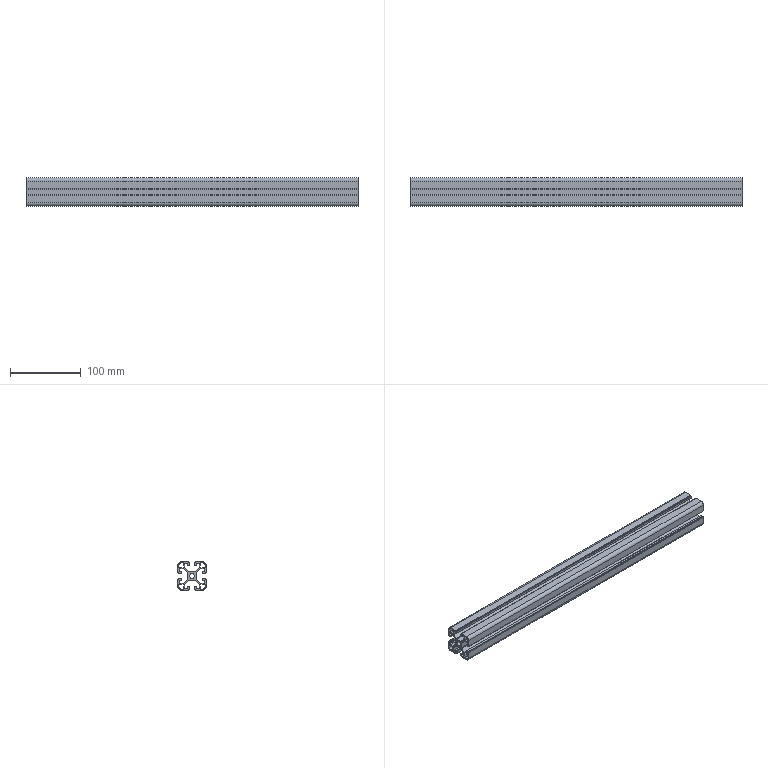Part | STEP file | MK-8-4040C-L-00 profile 4040C standard 470mm | 1 solid | 188 faces | box 470 x 40 x 40 mm | volume 224777 mm3 | cylinder 94 | plane 94 | commonest cylinder face diameters 0.6 x30 2 x28 4 x16 0.4 x8 6 x4 9 x4